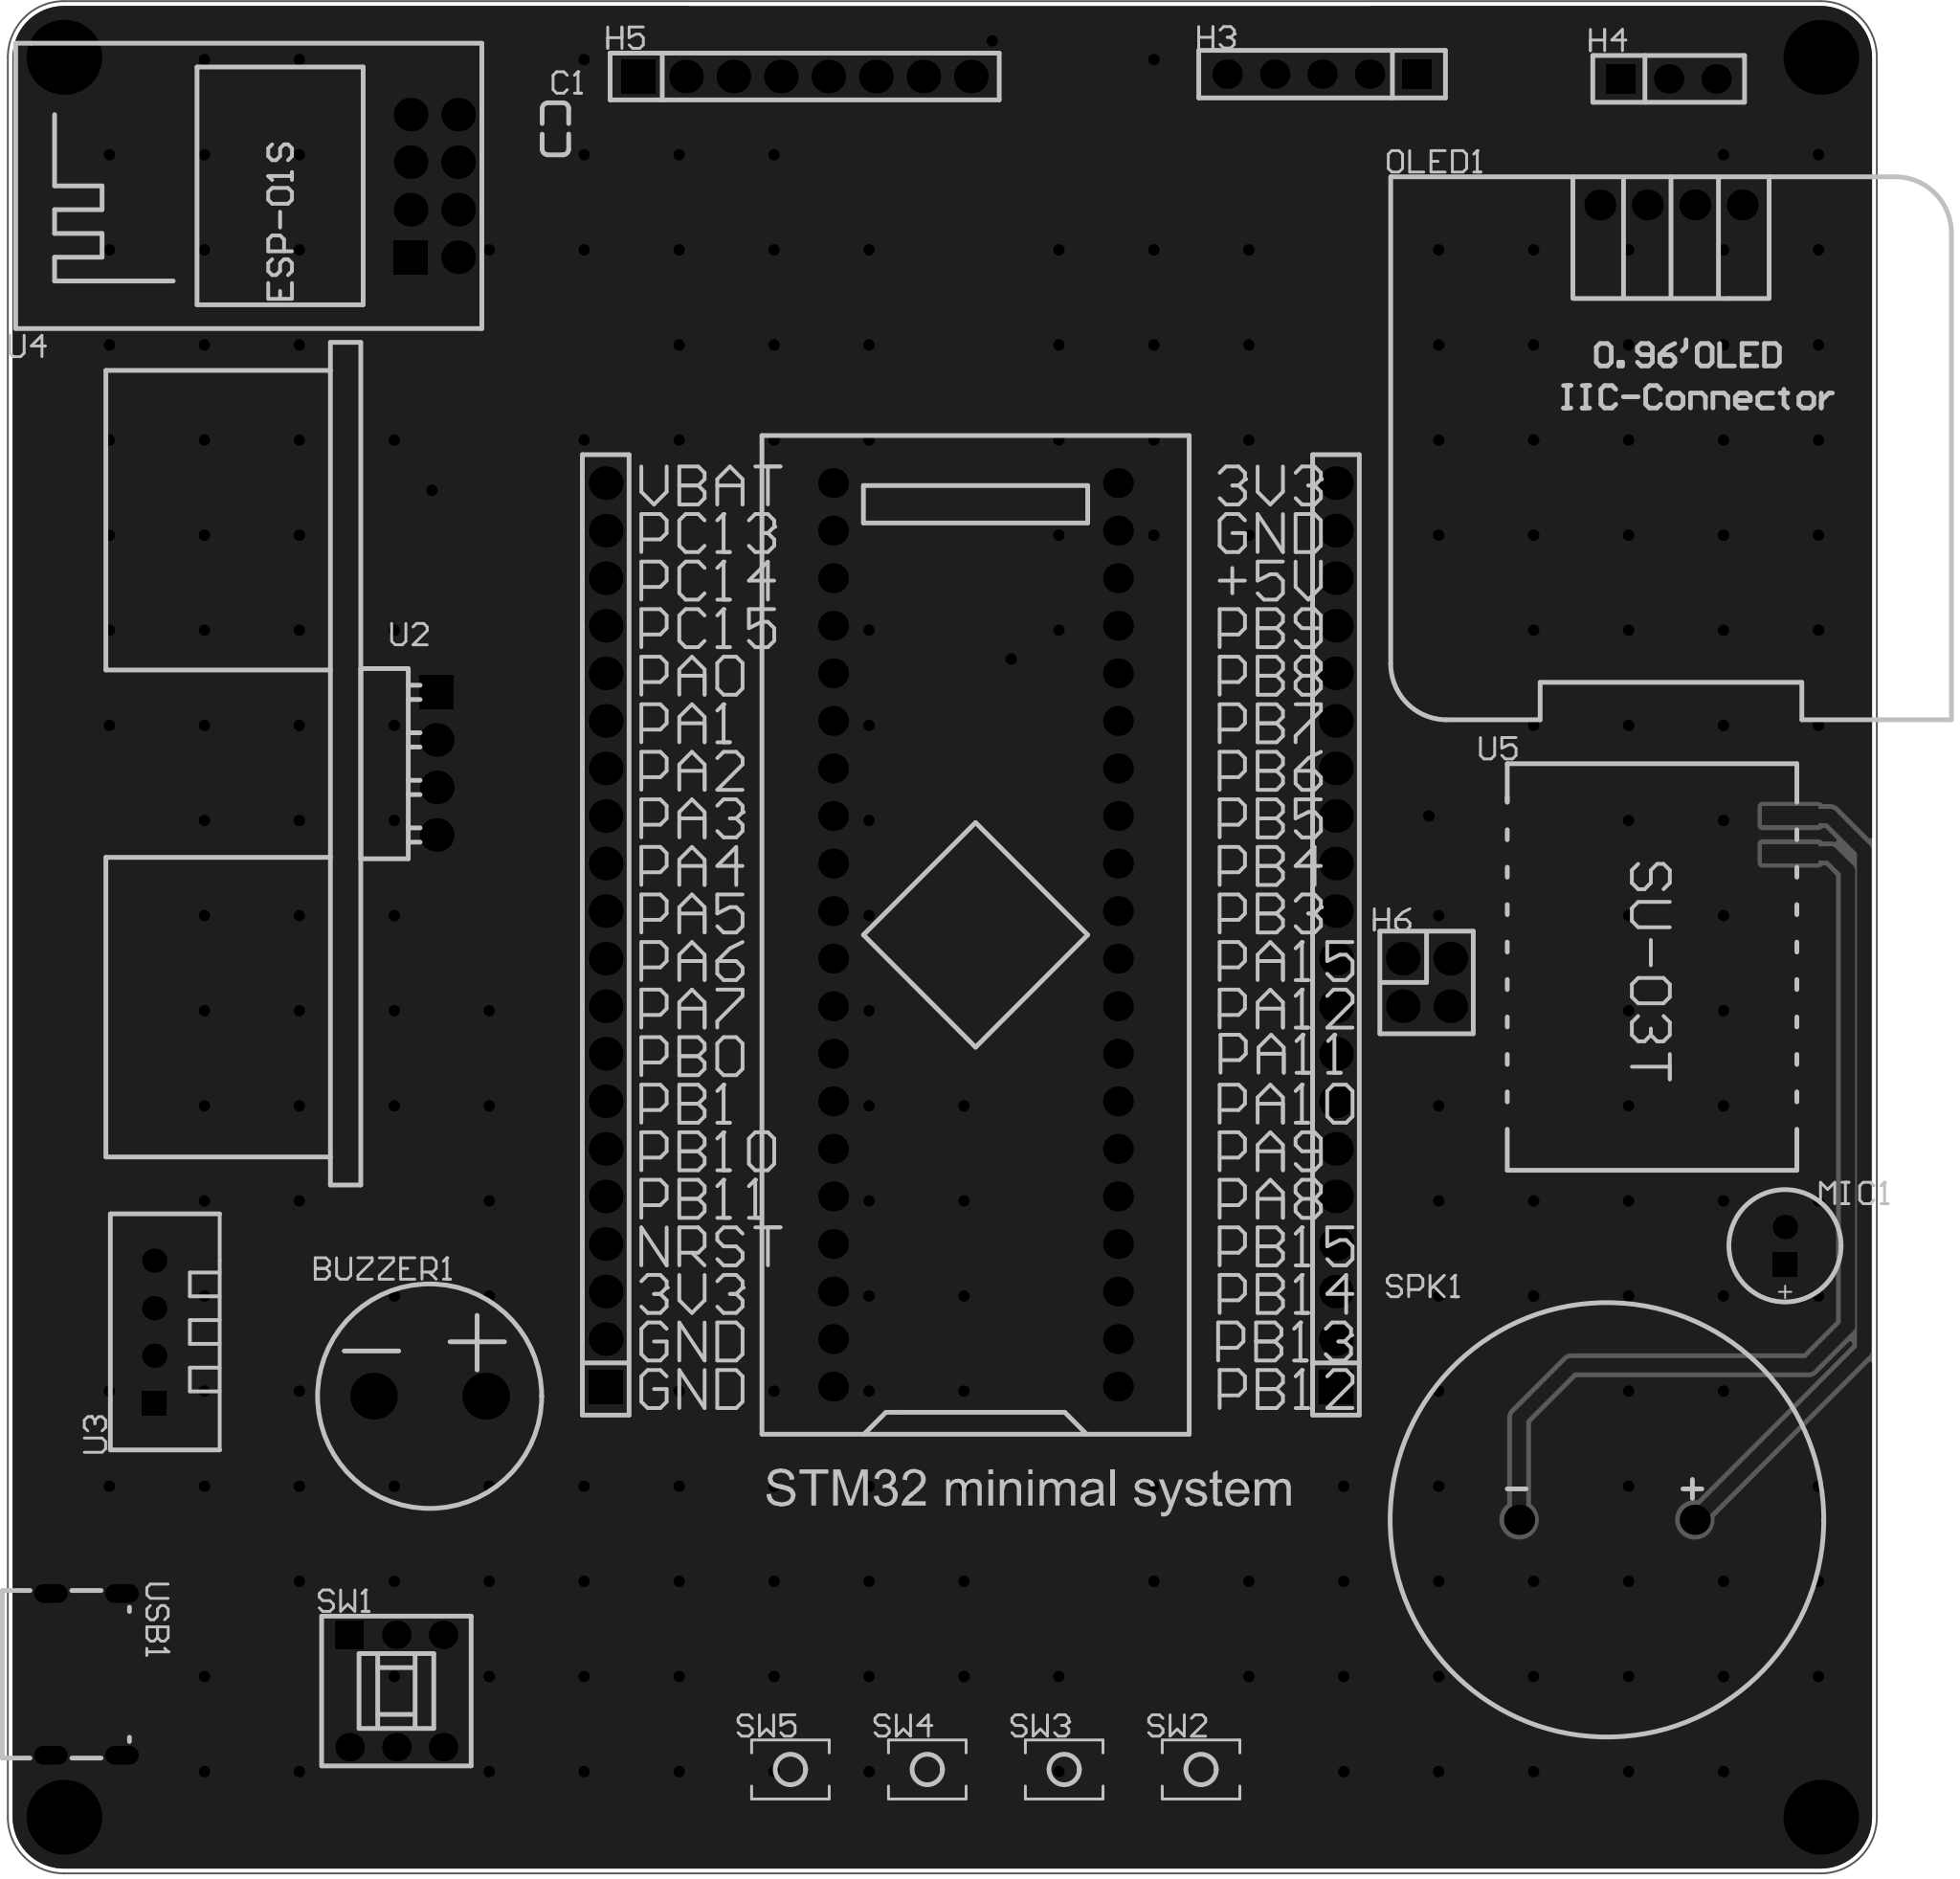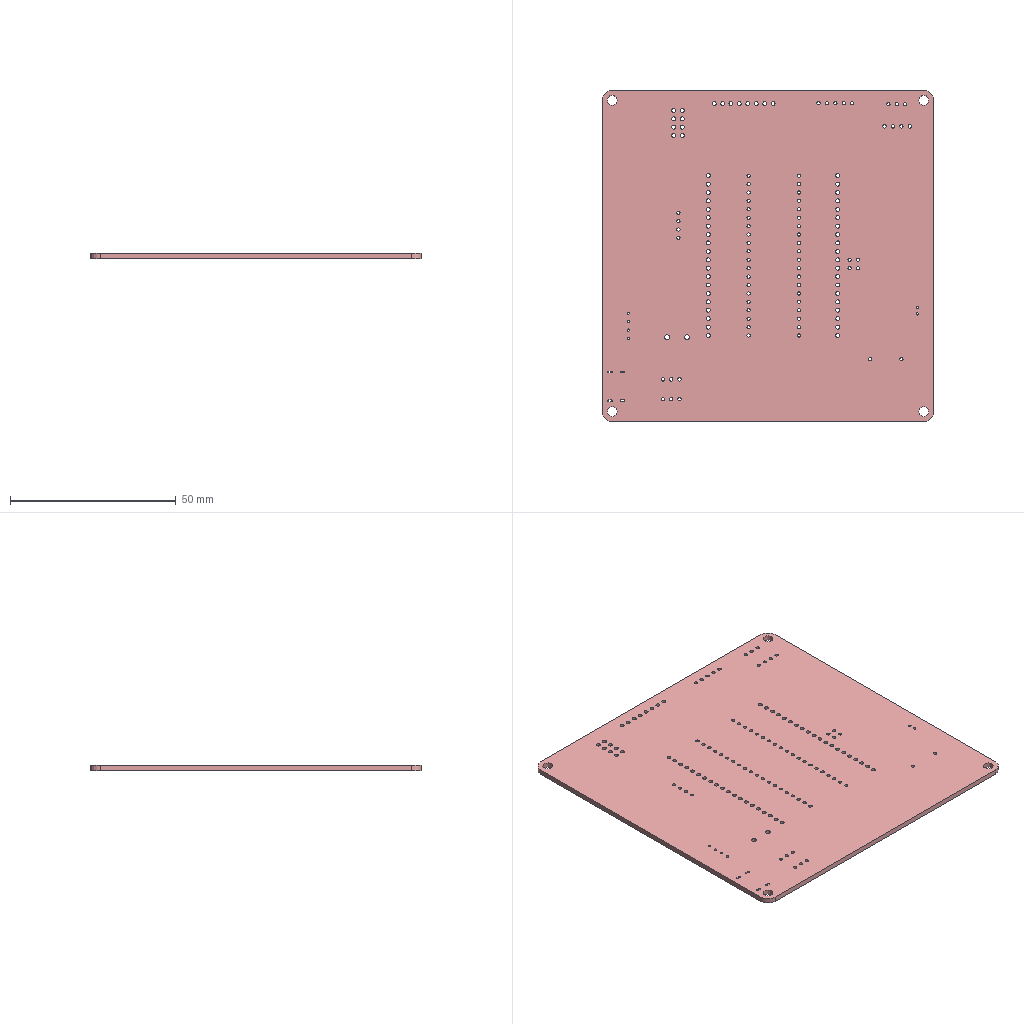Circuit board layout | Altium Designer | box 100 x 100 x 1.6 mm
Layer stack:
# Altium Designer layer stack of  (unit mm; dielectric type: 0 none, 1 core, 2 prepreg, 3 surface material)
index,name,kind,layer,copper_thickness_mm,dielectric_type,dielectric_thickness_mm,dielectric_material,dielectric_constant
0,Top Paste Mask Layer,other,,,,,,
1,Top Silkscreen Layer,other,,,,,,
2,Top Solder Mask Layer,dielectric,,,3,0.01,,3.3
3,Top Layer,copper,Top Layer,0.035,,,,
4,Dielectric1,dielectric,,,3,1.51,FR4,4.5
5,Bottom Layer,copper,Bottom Layer,0.035,,,,
6,Bottom Solder Mask Layer,dielectric,,,3,0.01,,3.3
7,Bottom Silkscreen Layer,other,,,,,,
8,Bottom Paste Mask Layer,other,,,,,,
# drill layer pairs: low layer,high layer
drill_pair,Top Layer,Bottom Layer
Part placement:
Designator,Comment,Layer,Footprint,Center-X(mm),Center-Y(mm),Rotation
U1,STM32F103C8T6-Card,TopLayer,CONN-TH_L53.3-W22.9_STM32F103C8T6-CARD,132.334,129.032,90
H1,,TopLayer,HDR-TH_20P-P2.54-V-F,151.617,129.032,90
H2,,TopLayer,HDR-TH_20P-P2.54-V-F,112.546,129.032,90
BUZZER1,Buz,TopLayer,BUZ-TH_BD12.0-P6.00-D0.9-RD,103.124,104.394,0
C1,100nF,TopLayer,C0603,109.855,172.085,270
H3,ATGM336H module,TopLayer,HDR-TH_5P-P2.54-V-F,150.876,175.006,180
H4,Vibration module,TopLayer,HDR-TH_3P-P2.54-V-F,169.418,174.752,0
H5,MPU6050,TopLayer,HDR-TH_8P-P2.54-V-F-1,123.19,174.879,0
H6,,TopLayer,HDR-TH_4P-P2.54-V-F-R2-C2-S2.54,156.464,126.492,270
MIC1,MIC,TopLayer,MIC-TH_BD6.0-P2.00,175.641,112.427,90
OLED1,,TopLayer,0.96OLED_4P,169.545,168.021,0
SPK1,FS-2308,TopLayer,BEEP-TH_BD23.2-P9.20-D1.0,166.116,97.79,0
SW1,PS081-06L135D1-JF-G,TopLayer,SW-TH_6P-L8.0-W8.0-P2.50-TL,101.346,88.646,0
SW2,,TopLayer,Key_SMD_3x4x2,144.399,84.455,0
SW3,,TopLayer,Key_SMD_3x4x2,137.075,84.455,0
SW4,,TopLayer,Key_SMD_3x4x2,129.752,84.455,0
SW5,,TopLayer,Key_SMD_3x4x2,122.428,84.455,0
U2,HC-SR04,TopLayer,TH_HC-SR04V,103.505,138.176,270
U3,DHT11 temperature and humidity,TopLayer,SENSOR-TH_DHT11,88.392,107.823,90
U4,ESP-01S,TopLayer,WIFIM-TH_ESP-01S,103.378,169.037,90
U5,SU-03T,TopLayer,COMM-SMD_18P-L21.0-W15.0-P2.00,168.529,127.381,0
USB1,TYPEC-250D-BCP6,TopLayer,USB-C-SMD_TYPEC-250D-BCP6,84.963,89.535,270
Pad and via stacks:
# Altium Designer via and pad stacks of  (unit mm). Each distinct definition once, with the count of objects using it.
# via: kind,start_layer,end_layer,hole_mm,diameter_mm,mode(0 simple;1 top-mid-bottom;2 full stack),diameter_per_layer,count,example_net
# pad: kind,layer,hole_mm,hole_type(0 round;1 square;2 slot),plating,top_size,top_shape(1 round;2 rect;3 octagon;9 rounded rect),mid_size,bottom_size,mode,footprint,size_per_layer,count,example
pad,Multi-Layer,3,0,plated,4x4,1,4x4,4x4,0,,,4,1
pad,Multi-Layer,1,0,plated,1.6x1.6,1,1.6x1.6,1.6x1.6,0,CONN-TH_L53.3-W22.9_STM32F103C8T6-CARD,,40,U1.1
pad,Multi-Layer,1.2,0,plated,1.8x1.8,2,1.8x1.8,1.8x1.8,0,HDR-TH_20P-P2.54-V-F,,2,H1.1
pad,Multi-Layer,1.2,0,plated,1.8x1.8,1,1.8x1.8,1.8x1.8,0,HDR-TH_20P-P2.54-V-F,,38,H1.2
pad,Multi-Layer,1.5,0,plated,2.5x2.5,1,2.5x2.5,2.5x2.5,0,BUZ-TH_BD12.0-P6.00-D0.9-RD,,2,BUZZER1.1
pad,Multi-Layer,1.02,0,plated,1.575x1.575,1,1.575x1.575,1.575x1.575,0,HDR-TH_5P-P2.54-V-F,,4,H3.5
pad,Multi-Layer,1.02,0,plated,1.575x1.575,2,1.575x1.575,1.575x1.575,0,HDR-TH_5P-P2.54-V-F,,1,H3.1
pad,Multi-Layer,1.02,0,plated,1.575x1.575,1,1.575x1.575,1.575x1.575,0,HDR-TH_3P-P2.54-V-F,,2,H4.3
pad,Multi-Layer,1.02,0,plated,1.575x1.575,2,1.575x1.575,1.575x1.575,0,HDR-TH_3P-P2.54-V-F,,1,H4.1
pad,Multi-Layer,1.2,0,plated,1.8x1.8,2,1.8x1.8,1.8x1.8,0,HDR-TH_8P-P2.54-V-F-1,,1,H5.1
pad,Multi-Layer,1.2,0,plated,1.8x1.8,1,1.8x1.8,1.8x1.8,0,HDR-TH_8P-P2.54-V-F-1,,7,H5.2
pad,Multi-Layer,1,0,plated,1.8x1.8,1,1.8x1.8,1.8x1.8,0,HDR-TH_4P-P2.54-V-F-R2-C2-S2.54,,4,H6.4
pad,Multi-Layer,0.7,0,plated,1.3x1.3,2,1.3x1.3,1.3x1.3,0,MIC-TH_BD6.0-P2.00,,1,MIC1.1
pad,Multi-Layer,0.7,0,plated,1.3x1.3,1,1.3x1.3,1.3x1.3,0,MIC-TH_BD6.0-P2.00,,1,MIC1.2
pad,Multi-Layer,1,0,plated,1.65x1.65,1,1.65x1.65,1.65x1.65,0,0.96OLED_4P,,4,OLED1.4
pad,Multi-Layer,1,0,plated,1.6x1.6,1,1.6x1.6,1.6x1.6,0,BEEP-TH_BD23.2-P9.20-D1.0,,2,SPK1.1
pad,Multi-Layer,1,0,plated,1.524x1.524,1,1.524x1.524,1.524x1.524,0,SW-TH_6P-L8.0-W8.0-P2.50-TL,,5,SW1.4
pad,Multi-Layer,1,0,plated,1.524x1.524,2,1.524x1.524,1.524x1.524,0,SW-TH_6P-L8.0-W8.0-P2.50-TL,,1,SW1.1
pad,Multi-Layer,1.001,0,plated,1.8x1.8,1,1.8x1.8,1.8x1.8,0,TH_HC-SR04V,,3,U2.4
pad,Multi-Layer,1.001,0,plated,1.8x1.8,2,1.8x1.8,1.8x1.8,0,TH_HC-SR04V,,1,U2.1
pad,Multi-Layer,0.7112,0,plated,1.295x1.295,2,1.295x1.295,1.295x1.295,0,SENSOR-TH_DHT11,,1,U3.1
pad,Multi-Layer,0.7112,0,plated,1.295x1.295,1,1.295x1.295,1.295x1.295,0,SENSOR-TH_DHT11,,3,U3.2
pad,Multi-Layer,1.2,0,plated,1.8x1.8,2,1.8x1.8,1.8x1.8,0,WIFIM-TH_ESP-01S,,1,U4.1
pad,Multi-Layer,1.2,0,plated,1.8x1.8,1,1.8x1.8,1.8x1.8,0,WIFIM-TH_ESP-01S,,7,U4.2
pad,Multi-Layer,0.5,2,plated,1x1.8,1,1x1.8,1x1.8,0,USB-C-SMD_TYPEC-250D-BCP6,,4,USB1.1
pad,Top Layer,0,0,plated,0.8x0.9,2,0.8x0.9,0.8x0.9,0,C0603,,2,C1.2
pad,Top Layer,0,0,plated,1.53x1.36,2,1.53x1.36,1.53x1.36,0,Key_SMD_3x4x2,,8,SW2.1
pad,Top Layer,0,0,plated,3x1,2,3x1,3x1,0,COMM-SMD_18P-L21.0-W15.0-P2.00,,18,U5.10
pad,Top Layer,0,0,plated,0.75x1.6,2,0.75x1.6,0.75x1.6,0,USB-C-SMD_TYPEC-250D-BCP6,,6,USB1.B12
via,Top Layer,Bottom Layer,0.3048,0.61,0,,212,PB5_MPUINT
Copper pours:
name,layer,net,type(0 solid;1 hatched;2 none)
Bottom Layer-GND,Bottom Layer,GND,0
Top Layer-GND,Top Layer,GND,0